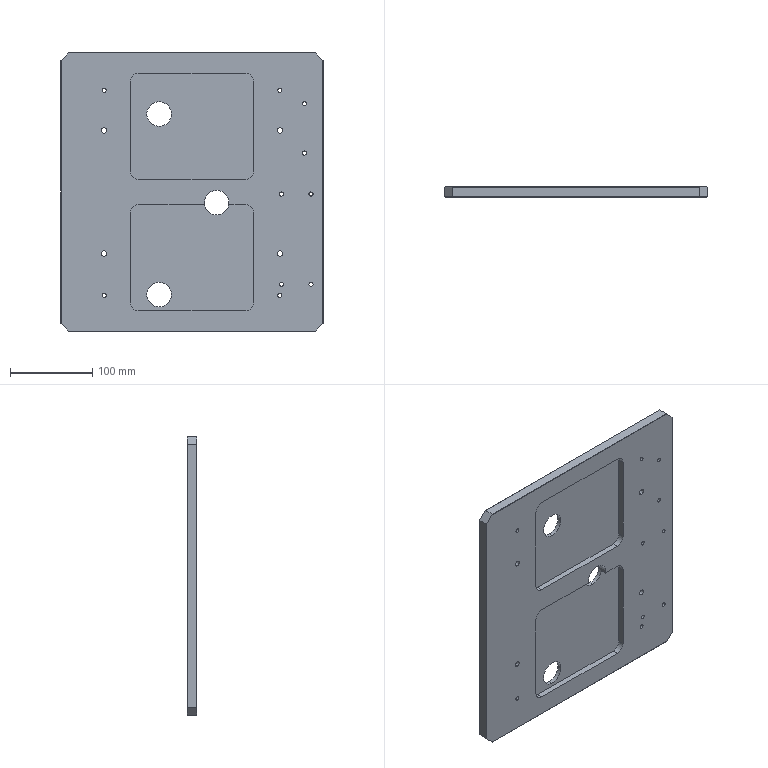Part | STEP file | 11-FG-SJ00511 | 1 solid | 83 faces | box 320 x 12 x 340 mm | volume 1012040 mm3 | cylinder 50 | plane 33 | commonest cylinder face diameters 5 x20 6.6 x8 11 x8 20 x8 30 x6